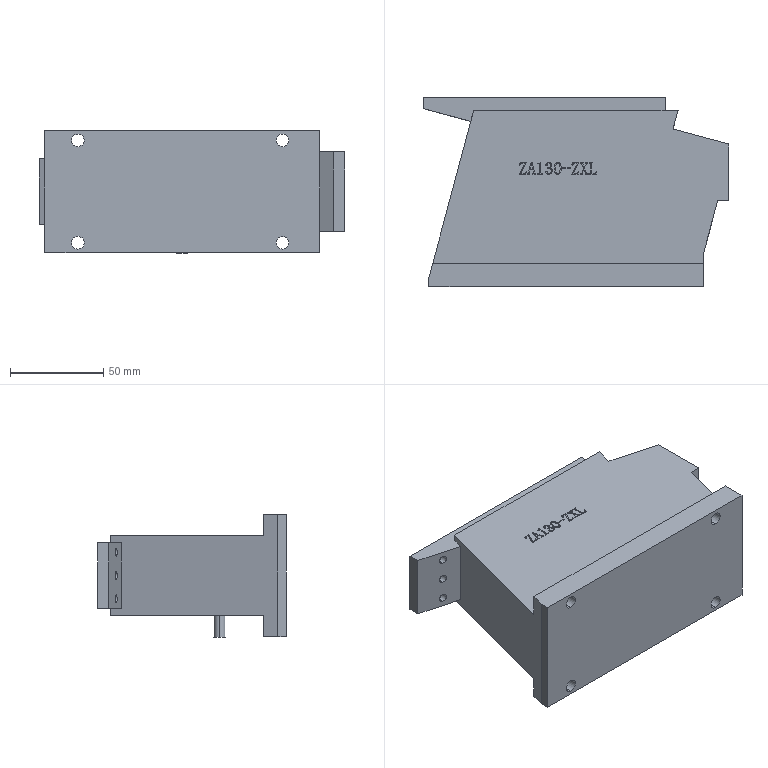Part | SolidWorks | features ICE 6, HoleWzd 2, Extrusion 1 | 1 solid | 229 faces | box 164 x 101.5 x 66 mm | volume 635286 mm3 | plane 131 | spline 58 | cylinder 28 | cone 12 | commonest cylinder face diameters 4.2 x18 6.8 x8 6 x2